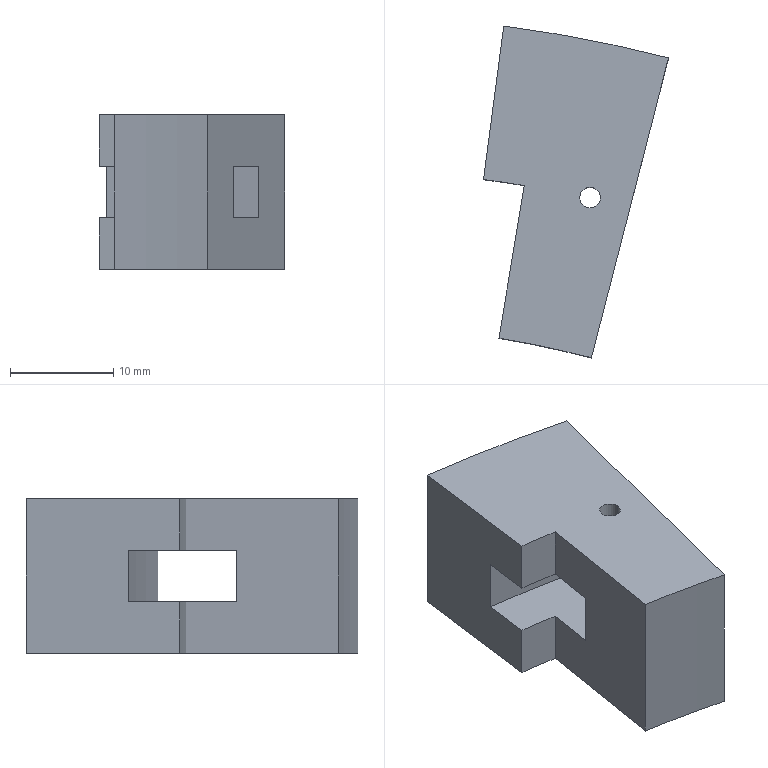Part | SolidWorks | features ICE 5, Extrusion 1 | 1 solid | 17 faces | box 17.933 x 32.148 x 15 mm | volume 5012 mm3 | cylinder 10 | plane 7 | commonest cylinder face diameters 2 x4 240 x2 210 x1 230 x1 249.998 x1 270 x1
STEP:
#1=CARTESIAN_POINT('',(24.989,117.22,0.));
#2=VERTEX_POINT('',#1);
#3=CARTESIAN_POINT('',(26.989,117.22,0.));
#4=VERTEX_POINT('',#3);
#5=CARTESIAN_POINT('',(25.989,117.22,0.));
#6=DIRECTION('',(0.,0.,1.));
#7=DIRECTION('',(1.,0.,0.));
#8=AXIS2_PLACEMENT_3D('',#5,#6,#7);
#9=CIRCLE('',#8,1.);
#10=EDGE_CURVE('',#2,#4,#9,.T.);
#11=ORIENTED_EDGE('',*,*,#10,.F.);
#12=CARTESIAN_POINT('',(24.989,117.22,5.));
#13=VERTEX_POINT('',#12);
#14=CARTESIAN_POINT('',(24.989,117.22,0.));
#15=DIRECTION('',(0.,0.,1.));
#16=VECTOR('',#15,1000.);
#17=LINE('',#14,#16);
#18=EDGE_CURVE('',#2,#13,#17,.T.);
#19=ORIENTED_EDGE('',*,*,#18,.T.);
#20=CARTESIAN_POINT('',(26.989,117.22,5.));
#21=VERTEX_POINT('',#20);
#22=CARTESIAN_POINT('',(25.989,117.22,5.));
#23=DIRECTION('',(0.,0.,1.));
#24=DIRECTION('',(1.,0.,0.));
#25=AXIS2_PLACEMENT_3D('',#22,#23,#24);
#26=CIRCLE('',#25,1.);
#27=EDGE_CURVE('',#13,#21,#26,.T.);
#28=ORIENTED_EDGE('',*,*,#27,.T.);
#29=CARTESIAN_POINT('',(26.989,117.22,0.));
#30=DIRECTION('',(0.,0.,1.));
#31=VECTOR('',#30,1000.);
#32=LINE('',#29,#31);
#33=EDGE_CURVE('',#4,#21,#32,.T.);
#34=ORIENTED_EDGE('',*,*,#33,.F.);
#35=EDGE_LOOP('',(#11,#19,#28,#34));
#36=FACE_OUTER_BOUND('',#35,.T.);
#37=CARTESIAN_POINT('',(25.989,117.22,0.));
#38=DIRECTION('',(0.,0.,1.));
#39=DIRECTION('',(1.,0.,0.));
#40=AXIS2_PLACEMENT_3D('',#37,#38,#39);
#41=CYLINDRICAL_SURFACE('',#40,1.);
#42=ADVANCED_FACE('',(#36),#41,.F.);
#43=CARTESIAN_POINT('',(24.989,117.22,10.));
#44=VERTEX_POINT('',#43);
#45=CARTESIAN_POINT('',(26.989,117.22,10.));
#46=VERTEX_POINT('',#45);
#47=CARTESIAN_POINT('',(25.989,117.22,10.));
#48=DIRECTION('',(0.,0.,1.));
#49=DIRECTION('',(1.,0.,0.));
#50=AXIS2_PLACEMENT_3D('',#47,#48,#49);
#51=CIRCLE('',#50,1.);
#52=EDGE_CURVE('',#44,#46,#51,.T.);
#53=ORIENTED_EDGE('',*,*,#52,.F.);
#54=CARTESIAN_POINT('',(24.989,117.22,15.));
#55=VERTEX_POINT('',#54);
#56=CARTESIAN_POINT('',(24.989,117.22,0.));
#57=DIRECTION('',(0.,0.,1.));
#58=VECTOR('',#57,1000.);
#59=LINE('',#56,#58);
#60=EDGE_CURVE('',#44,#55,#59,.T.);
#61=ORIENTED_EDGE('',*,*,#60,.T.);
#62=CARTESIAN_POINT('',(26.989,117.22,15.));
#63=VERTEX_POINT('',#62);
#64=CARTESIAN_POINT('',(25.989,117.22,15.));
#65=DIRECTION('',(0.,0.,1.));
#66=DIRECTION('',(1.,0.,0.));
#67=AXIS2_PLACEMENT_3D('',#64,#65,#66);
#68=CIRCLE('',#67,1.);
#69=EDGE_CURVE('',#55,#63,#68,.T.);
#70=ORIENTED_EDGE('',*,*,#69,.T.);
#71=CARTESIAN_POINT('',(26.989,117.22,0.));
#72=DIRECTION('',(0.,0.,1.));
#73=VECTOR('',#72,1000.);
#74=LINE('',#71,#73);
#75=EDGE_CURVE('',#46,#63,#74,.T.);
#76=ORIENTED_EDGE('',*,*,#75,.F.);
#77=EDGE_LOOP('',(#53,#61,#70,#76));
#78=FACE_OUTER_BOUND('',#77,.T.);
#79=CARTESIAN_POINT('',(25.989,117.22,0.));
#80=DIRECTION('',(0.,0.,1.));
#81=DIRECTION('',(1.,0.,0.));
#82=AXIS2_PLACEMENT_3D('',#79,#80,#81);
#83=CYLINDRICAL_SURFACE('',#82,1.);
#84=ADVANCED_FACE('',(#78),#83,.F.);
#85=CARTESIAN_POINT('',(28.619,111.382,10.));
#86=VERTEX_POINT('',#85);
#87=CARTESIAN_POINT('',(18.802,113.453,10.));
#88=VERTEX_POINT('',#87);
#89=CARTESIAN_POINT('',(0.,0.,10.));
#90=DIRECTION('',(0.,0.,1.));
#91=DIRECTION('',(1.,0.,0.));
#92=AXIS2_PLACEMENT_3D('',#89,#90,#91);
#93=CIRCLE('',#92,115.);
#94=EDGE_CURVE('',#86,#88,#93,.T.);
#95=ORIENTED_EDGE('',*,*,#94,.F.);
#96=CARTESIAN_POINT('',(28.619,111.382,5.));
#97=VERTEX_POINT('',#96);
#98=CARTESIAN_POINT('',(28.619,111.382,5.));
#99=DIRECTION('',(0.,0.,1.));
#100=VECTOR('',#99,1000.);
#101=LINE('',#98,#100);
#102=EDGE_CURVE('',#97,#86,#101,.T.);
#103=ORIENTED_EDGE('',*,*,#102,.F.);
#104=CARTESIAN_POINT('',(18.802,113.453,5.));
#105=VERTEX_POINT('',#104);
#106=CARTESIAN_POINT('',(0.,0.,5.));
#107=DIRECTION('',(0.,0.,-1.));
#108=DIRECTION('',(1.,0.,0.));
#109=AXIS2_PLACEMENT_3D('',#106,#107,#108);
#110=CIRCLE('',#109,115.);
#111=EDGE_CURVE('',#105,#97,#110,.T.);
#112=ORIENTED_EDGE('',*,*,#111,.F.);
#113=CARTESIAN_POINT('',(18.802,113.453,15.));
#114=DIRECTION('',(0.,0.,-1.));
#115=VECTOR('',#114,1000.);
#116=LINE('',#113,#115);
#117=EDGE_CURVE('',#88,#105,#116,.T.);
#118=ORIENTED_EDGE('',*,*,#117,.F.);
#119=EDGE_LOOP('',(#95,#103,#112,#118));
#120=FACE_OUTER_BOUND('',#119,.T.);
#121=CARTESIAN_POINT('',(0.,0.,5.));
#122=DIRECTION('',(0.,0.,1.));
#123=DIRECTION('',(1.,0.,0.));
#124=AXIS2_PLACEMENT_3D('',#121,#122,#123);
#125=CYLINDRICAL_SURFACE('',#124,115.);
#126=ADVANCED_FACE('',(#120),#125,.T.);
#127=CARTESIAN_POINT('',(16.316,123.93,5.));
#128=VERTEX_POINT('',#127);
#129=CARTESIAN_POINT('',(16.316,123.93,10.));
#130=VERTEX_POINT('',#129);
#131=CARTESIAN_POINT('',(16.316,123.93,5.));
#132=DIRECTION('',(0.,0.,1.));
#133=VECTOR('',#132,1000.);
#134=LINE('',#131,#133);
#135=EDGE_CURVE('',#128,#130,#134,.T.);
#136=ORIENTED_EDGE('',*,*,#135,.F.);
#137=CARTESIAN_POINT('',(31.107,121.067,5.));
#138=VERTEX_POINT('',#137);
#139=CARTESIAN_POINT('',(0.,0.,5.));
#140=DIRECTION('',(0.,0.,-1.));
#141=DIRECTION('',(1.,0.,0.));
#142=AXIS2_PLACEMENT_3D('',#139,#140,#141);
#143=CIRCLE('',#142,124.999);
#144=EDGE_CURVE('',#128,#138,#143,.T.);
#145=ORIENTED_EDGE('',*,*,#144,.T.);
#146=CARTESIAN_POINT('',(31.107,121.067,10.));
#147=VERTEX_POINT('',#146);
#148=CARTESIAN_POINT('',(31.107,121.067,5.));
#149=DIRECTION('',(0.,0.,1.));
#150=VECTOR('',#149,1000.);
#151=LINE('',#148,#150);
#152=EDGE_CURVE('',#138,#147,#151,.T.);
#153=ORIENTED_EDGE('',*,*,#152,.T.);
#154=CARTESIAN_POINT('',(0.,0.,10.));
#155=DIRECTION('',(0.,0.,-1.));
#156=DIRECTION('',(1.,0.,0.));
#157=AXIS2_PLACEMENT_3D('',#154,#155,#156);
#158=CIRCLE('',#157,124.999);
#159=EDGE_CURVE('',#130,#147,#158,.T.);
#160=ORIENTED_EDGE('',*,*,#159,.F.);
#161=EDGE_LOOP('',(#136,#145,#153,#160));
#162=FACE_OUTER_BOUND('',#161,.T.);
#163=CARTESIAN_POINT('',(0.,0.,5.));
#164=DIRECTION('',(0.,0.,1.));
#165=DIRECTION('',(1.,0.,0.));
#166=AXIS2_PLACEMENT_3D('',#163,#164,#165);
#167=CYLINDRICAL_SURFACE('',#166,124.999);
#168=ADVANCED_FACE('',(#162),#167,.F.);
#169=CARTESIAN_POINT('',(33.596,130.753,15.));
#170=VERTEX_POINT('',#169);
#171=CARTESIAN_POINT('',(33.596,130.753,0.));
#172=VERTEX_POINT('',#171);
#173=CARTESIAN_POINT('',(33.596,130.753,15.));
#174=DIRECTION('',(0.,0.,-1.));
#175=VECTOR('',#174,1000.);
#176=LINE('',#173,#175);
#177=EDGE_CURVE('',#170,#172,#176,.T.);
#178=ORIENTED_EDGE('',*,*,#177,.F.);
#179=CARTESIAN_POINT('',(26.13,101.697,15.));
#180=VERTEX_POINT('',#179);
#181=CARTESIAN_POINT('',(26.13,101.697,15.));
#182=DIRECTION('',(0.2489,0.9685,0.));
#183=VECTOR('',#182,1000.);
#184=LINE('',#181,#183);
#185=EDGE_CURVE('',#180,#170,#184,.T.);
#186=ORIENTED_EDGE('',*,*,#185,.F.);
#187=CARTESIAN_POINT('',(26.13,101.697,0.));
#188=VERTEX_POINT('',#187);
#189=CARTESIAN_POINT('',(26.13,101.697,15.));
#190=DIRECTION('',(0.,0.,-1.));
#191=VECTOR('',#190,1000.);
#192=LINE('',#189,#191);
#193=EDGE_CURVE('',#180,#188,#192,.T.);
#194=ORIENTED_EDGE('',*,*,#193,.T.);
#195=CARTESIAN_POINT('',(26.13,101.697,0.));
#196=DIRECTION('',(0.2489,0.9685,0.));
#197=VECTOR('',#196,1000.);
#198=LINE('',#195,#197);
#199=EDGE_CURVE('',#188,#172,#198,.T.);
#200=ORIENTED_EDGE('',*,*,#199,.T.);
#201=EDGE_LOOP('',(#178,#186,#194,#200));
#202=FACE_OUTER_BOUND('',#201,.T.);
#203=ORIENTED_EDGE('',*,*,#152,.F.);
#204=CARTESIAN_POINT('',(0.,0.,5.));
#205=DIRECTION('',(0.2489,0.9685,0.));
#206=VECTOR('',#205,1000.);
#207=LINE('',#204,#206);
#208=EDGE_CURVE('',#97,#138,#207,.T.);
#209=ORIENTED_EDGE('',*,*,#208,.F.);
#210=ORIENTED_EDGE('',*,*,#102,.T.);
#211=CARTESIAN_POINT('',(0.,0.,10.));
#212=DIRECTION('',(0.2489,0.9685,0.));
#213=VECTOR('',#212,1000.);
#214=LINE('',#211,#213);
#215=EDGE_CURVE('',#86,#147,#214,.T.);
#216=ORIENTED_EDGE('',*,*,#215,.T.);
#217=EDGE_LOOP('',(#203,#209,#210,#216));
#218=FACE_BOUND('',#217,.T.);
#219=CARTESIAN_POINT('',(26.13,101.697,15.));
#220=DIRECTION('',(-0.9685,0.2489,0.));
#221=DIRECTION('',(-0.2489,-0.9685,0.));
#222=AXIS2_PLACEMENT_3D('',#219,#220,#221);
#223=PLANE('',#222);
#224=ADVANCED_FACE('',(#202,#218),#223,.F.);
#225=CARTESIAN_POINT('',(17.621,133.845,0.));
#226=VERTEX_POINT('',#225);
#227=CARTESIAN_POINT('',(0.,0.,0.));
#228=DIRECTION('',(0.,0.,1.));
#229=DIRECTION('',(1.,0.,0.));
#230=AXIS2_PLACEMENT_3D('',#227,#228,#229);
#231=CIRCLE('',#230,135.);
#232=EDGE_CURVE('',#172,#226,#231,.T.);
#233=ORIENTED_EDGE('',*,*,#232,.T.);
#234=CARTESIAN_POINT('',(17.621,133.845,15.));
#235=VERTEX_POINT('',#234);
#236=CARTESIAN_POINT('',(17.621,133.845,0.));
#237=DIRECTION('',(0.,0.,1.));
#238=VECTOR('',#237,1000.);
#239=LINE('',#236,#238);
#240=EDGE_CURVE('',#226,#235,#239,.T.);
#241=ORIENTED_EDGE('',*,*,#240,.T.);
#242=CARTESIAN_POINT('',(0.,0.,15.));
#243=DIRECTION('',(0.,0.,1.));
#244=DIRECTION('',(1.,0.,0.));
#245=AXIS2_PLACEMENT_3D('',#242,#243,#244);
#246=CIRCLE('',#245,135.);
#247=EDGE_CURVE('',#170,#235,#246,.T.);
#248=ORIENTED_EDGE('',*,*,#247,.F.);
#249=ORIENTED_EDGE('',*,*,#177,.T.);
#250=EDGE_LOOP('',(#233,#241,#248,#249));
#251=FACE_OUTER_BOUND('',#250,.T.);
#252=CARTESIAN_POINT('',(0.,0.,15.));
#253=DIRECTION('',(0.,0.,-1.));
#254=DIRECTION('',(-1.,0.,0.));
#255=AXIS2_PLACEMENT_3D('',#252,#253,#254);
#256=CYLINDRICAL_SURFACE('',#255,135.);
#257=ADVANCED_FACE('',(#251),#256,.T.);
#258=CARTESIAN_POINT('',(19.62,118.385,0.));
#259=VERTEX_POINT('',#258);
#260=CARTESIAN_POINT('',(17.167,103.587,0.));
#261=VERTEX_POINT('',#260);
#262=CARTESIAN_POINT('',(17.167,103.587,0.));
#263=DIRECTION('',(-0.1635,-0.9865,0.));
#264=VECTOR('',#263,1000.);
#265=LINE('',#262,#264);
#266=EDGE_CURVE('',#259,#261,#265,.T.);
#267=ORIENTED_EDGE('',*,*,#266,.T.);
#268=CARTESIAN_POINT('',(17.167,103.587,15.));
#269=VERTEX_POINT('',#268);
#270=CARTESIAN_POINT('',(17.167,103.587,15.));
#271=DIRECTION('',(0.,0.,-1.));
#272=VECTOR('',#271,1000.);
#273=LINE('',#270,#272);
#274=EDGE_CURVE('',#269,#261,#273,.T.);
#275=ORIENTED_EDGE('',*,*,#274,.F.);
#276=CARTESIAN_POINT('',(19.62,118.385,15.));
#277=VERTEX_POINT('',#276);
#278=CARTESIAN_POINT('',(17.167,103.587,15.));
#279=DIRECTION('',(-0.1635,-0.9865,0.));
#280=VECTOR('',#279,1000.);
#281=LINE('',#278,#280);
#282=EDGE_CURVE('',#277,#269,#281,.T.);
#283=ORIENTED_EDGE('',*,*,#282,.F.);
#284=CARTESIAN_POINT('',(19.62,118.385,10.));
#285=VERTEX_POINT('',#284);
#286=CARTESIAN_POINT('',(19.62,118.385,0.));
#287=DIRECTION('',(0.,0.,1.));
#288=VECTOR('',#287,1000.);
#289=LINE('',#286,#288);
#290=EDGE_CURVE('',#285,#277,#289,.T.);
#291=ORIENTED_EDGE('',*,*,#290,.F.);
#292=CARTESIAN_POINT('',(0.,0.,10.));
#293=DIRECTION('',(0.1635,0.9865,0.));
#294=VECTOR('',#293,1000.);
#295=LINE('',#292,#294);
#296=EDGE_CURVE('',#88,#285,#295,.T.);
#297=ORIENTED_EDGE('',*,*,#296,.F.);
#298=ORIENTED_EDGE('',*,*,#117,.T.);
#299=CARTESIAN_POINT('',(19.62,118.385,5.));
#300=VERTEX_POINT('',#299);
#301=CARTESIAN_POINT('',(0.,0.,5.));
#302=DIRECTION('',(0.1635,0.9865,0.));
#303=VECTOR('',#302,1000.);
#304=LINE('',#301,#303);
#305=EDGE_CURVE('',#105,#300,#304,.T.);
#306=ORIENTED_EDGE('',*,*,#305,.T.);
#307=CARTESIAN_POINT('',(19.62,118.385,0.));
#308=DIRECTION('',(0.,0.,1.));
#309=VECTOR('',#308,1000.);
#310=LINE('',#307,#309);
#311=EDGE_CURVE('',#259,#300,#310,.T.);
#312=ORIENTED_EDGE('',*,*,#311,.F.);
#313=EDGE_LOOP('',(#267,#275,#283,#291,#297,#298,#306,#312));
#314=FACE_OUTER_BOUND('',#313,.T.);
#315=CARTESIAN_POINT('',(17.167,103.587,15.));
#316=DIRECTION('',(0.9865,-0.1635,0.));
#317=DIRECTION('',(0.1635,0.9865,0.));
#318=AXIS2_PLACEMENT_3D('',#315,#316,#317);
#319=PLANE('',#318);
#320=ADVANCED_FACE('',(#314),#319,.F.);
#321=CARTESIAN_POINT('',(0.,0.,0.));
#322=DIRECTION('',(0.,0.,-1.));
#323=DIRECTION('',(1.,0.,0.));
#324=AXIS2_PLACEMENT_3D('',#321,#322,#323);
#325=CIRCLE('',#324,105.);
#326=EDGE_CURVE('',#261,#188,#325,.T.);
#327=ORIENTED_EDGE('',*,*,#326,.T.);
#328=ORIENTED_EDGE('',*,*,#193,.F.);
#329=CARTESIAN_POINT('',(0.,0.,15.));
#330=DIRECTION('',(0.,0.,-1.));
#331=DIRECTION('',(1.,0.,0.));
#332=AXIS2_PLACEMENT_3D('',#329,#330,#331);
#333=CIRCLE('',#332,105.);
#334=EDGE_CURVE('',#269,#180,#333,.T.);
#335=ORIENTED_EDGE('',*,*,#334,.F.);
#336=ORIENTED_EDGE('',*,*,#274,.T.);
#337=EDGE_LOOP('',(#327,#328,#335,#336));
#338=FACE_OUTER_BOUND('',#337,.T.);
#339=CARTESIAN_POINT('',(0.,0.,15.));
#340=DIRECTION('',(0.,0.,-1.));
#341=DIRECTION('',(-1.,0.,0.));
#342=AXIS2_PLACEMENT_3D('',#339,#340,#341);
#343=CYLINDRICAL_SURFACE('',#342,105.);
#344=ADVANCED_FACE('',(#338),#343,.F.);
#345=CARTESIAN_POINT('',(15.663,118.973,15.));
#346=VERTEX_POINT('',#345);
#347=CARTESIAN_POINT('',(0.,0.,15.));
#348=DIRECTION('',(0.,0.,1.));
#349=DIRECTION('',(1.,0.,0.));
#350=AXIS2_PLACEMENT_3D('',#347,#348,#349);
#351=CIRCLE('',#350,120.);
#352=EDGE_CURVE('',#277,#346,#351,.T.);
#353=ORIENTED_EDGE('',*,*,#352,.F.);
#354=ORIENTED_EDGE('',*,*,#282,.T.);
#355=ORIENTED_EDGE('',*,*,#334,.T.);
#356=ORIENTED_EDGE('',*,*,#185,.T.);
#357=ORIENTED_EDGE('',*,*,#247,.T.);
#358=CARTESIAN_POINT('',(15.011,114.016,15.));
#359=DIRECTION('',(0.1305,0.9914,0.));
#360=VECTOR('',#359,1000.);
#361=LINE('',#358,#360);
#362=EDGE_CURVE('',#346,#235,#361,.T.);
#363=ORIENTED_EDGE('',*,*,#362,.F.);
#364=EDGE_LOOP('',(#353,#354,#355,#356,#357,#363));
#365=FACE_OUTER_BOUND('',#364,.T.);
#366=CARTESIAN_POINT('',(25.989,117.22,15.));
#367=DIRECTION('',(0.,0.,1.));
#368=DIRECTION('',(1.,0.,0.));
#369=AXIS2_PLACEMENT_3D('',#366,#367,#368);
#370=CIRCLE('',#369,1.);
#371=EDGE_CURVE('',#63,#55,#370,.T.);
#372=ORIENTED_EDGE('',*,*,#371,.F.);
#373=ORIENTED_EDGE('',*,*,#69,.F.);
#374=EDGE_LOOP('',(#372,#373));
#375=FACE_BOUND('',#374,.T.);
#376=CARTESIAN_POINT('',(0.,0.,15.));
#377=DIRECTION('',(0.,0.,1.));
#378=DIRECTION('',(1.,0.,0.));
#379=AXIS2_PLACEMENT_3D('',#376,#377,#378);
#380=PLANE('',#379);
#381=ADVANCED_FACE('',(#365,#375),#380,.T.);
#382=CARTESIAN_POINT('',(25.989,117.22,0.));
#383=DIRECTION('',(0.,0.,1.));
#384=DIRECTION('',(1.,0.,0.));
#385=AXIS2_PLACEMENT_3D('',#382,#383,#384);
#386=CIRCLE('',#385,1.);
#387=EDGE_CURVE('',#4,#2,#386,.T.);
#388=ORIENTED_EDGE('',*,*,#387,.T.);
#389=ORIENTED_EDGE('',*,*,#10,.T.);
#390=EDGE_LOOP('',(#388,#389));
#391=FACE_BOUND('',#390,.T.);
#392=ORIENTED_EDGE('',*,*,#266,.F.);
#393=CARTESIAN_POINT('',(15.663,118.973,0.));
#394=VERTEX_POINT('',#393);
#395=CARTESIAN_POINT('',(0.,0.,0.));
#396=DIRECTION('',(0.,0.,1.));
#397=DIRECTION('',(1.,0.,0.));
#398=AXIS2_PLACEMENT_3D('',#395,#396,#397);
#399=CIRCLE('',#398,120.);
#400=EDGE_CURVE('',#259,#394,#399,.T.);
#401=ORIENTED_EDGE('',*,*,#400,.T.);
#402=CARTESIAN_POINT('',(15.011,114.016,0.));
#403=DIRECTION('',(0.1305,0.9914,0.));
#404=VECTOR('',#403,1000.);
#405=LINE('',#402,#404);
#406=EDGE_CURVE('',#394,#226,#405,.T.);
#407=ORIENTED_EDGE('',*,*,#406,.T.);
#408=ORIENTED_EDGE('',*,*,#232,.F.);
#409=ORIENTED_EDGE('',*,*,#199,.F.);
#410=ORIENTED_EDGE('',*,*,#326,.F.);
#411=EDGE_LOOP('',(#392,#401,#407,#408,#409,#410));
#412=FACE_OUTER_BOUND('',#411,.T.);
#413=CARTESIAN_POINT('',(0.,0.,0.));
#414=DIRECTION('',(0.,0.,1.));
#415=DIRECTION('',(1.,0.,0.));
#416=AXIS2_PLACEMENT_3D('',#413,#414,#415);
#417=PLANE('',#416);
#418=ADVANCED_FACE('',(#391,#412),#417,.F.);
#419=CARTESIAN_POINT('',(15.663,118.973,5.));
#420=VERTEX_POINT('',#419);
#421=CARTESIAN_POINT('',(0.,0.,5.));
#422=DIRECTION('',(0.,0.,1.));
#423=DIRECTION('',(1.,0.,0.));
#424=AXIS2_PLACEMENT_3D('',#421,#422,#423);
#425=CIRCLE('',#424,120.);
#426=EDGE_CURVE('',#300,#420,#425,.T.);
#427=ORIENTED_EDGE('',*,*,#426,.F.);
#428=ORIENTED_EDGE('',*,*,#305,.F.);
#429=ORIENTED_EDGE('',*,*,#111,.T.);
#430=ORIENTED_EDGE('',*,*,#208,.T.);
#431=ORIENTED_EDGE('',*,*,#144,.F.);
#432=CARTESIAN_POINT('',(0.,0.,5.));
#433=DIRECTION('',(0.1305,0.9914,0.));
#434=VECTOR('',#433,1000.);
#435=LINE('',#432,#434);
#436=EDGE_CURVE('',#420,#128,#435,.T.);
#437=ORIENTED_EDGE('',*,*,#436,.F.);
#438=EDGE_LOOP('',(#427,#428,#429,#430,#431,#437));
#439=FACE_OUTER_BOUND('',#438,.T.);
#440=CARTESIAN_POINT('',(25.989,117.22,5.));
#441=DIRECTION('',(0.,0.,1.));
#442=DIRECTION('',(1.,0.,0.));
#443=AXIS2_PLACEMENT_3D('',#440,#441,#442);
#444=CIRCLE('',#443,1.);
#445=EDGE_CURVE('',#21,#13,#444,.T.);
#446=ORIENTED_EDGE('',*,*,#445,.F.);
#447=ORIENTED_EDGE('',*,*,#27,.F.);
#448=EDGE_LOOP('',(#446,#447));
#449=FACE_BOUND('',#448,.T.);
#450=CARTESIAN_POINT('',(0.,0.,5.));
#451=DIRECTION('',(0.,0.,1.));
#452=DIRECTION('',(1.,0.,0.));
#453=AXIS2_PLACEMENT_3D('',#450,#451,#452);
#454=PLANE('',#453);
#455=ADVANCED_FACE('',(#439,#449),#454,.T.);
#456=CARTESIAN_POINT('',(25.989,117.22,10.));
#457=DIRECTION('',(0.,0.,1.));
#458=DIRECTION('',(1.,0.,0.));
#459=AXIS2_PLACEMENT_3D('',#456,#457,#458);
#460=CIRCLE('',#459,1.);
#461=EDGE_CURVE('',#46,#44,#460,.T.);
#462=ORIENTED_EDGE('',*,*,#461,.T.);
#463=ORIENTED_EDGE('',*,*,#52,.T.);
#464=EDGE_LOOP('',(#462,#463));
#465=FACE_BOUND('',#464,.T.);
#466=ORIENTED_EDGE('',*,*,#296,.T.);
#467=CARTESIAN_POINT('',(15.663,118.973,10.));
#468=VERTEX_POINT('',#467);
#469=CARTESIAN_POINT('',(0.,0.,10.));
#470=DIRECTION('',(0.,0.,1.));
#471=DIRECTION('',(1.,0.,0.));
#472=AXIS2_PLACEMENT_3D('',#469,#470,#471);
#473=CIRCLE('',#472,120.);
#474=EDGE_CURVE('',#285,#468,#473,.T.);
#475=ORIENTED_EDGE('',*,*,#474,.T.);
#476=CARTESIAN_POINT('',(0.,0.,10.));
#477=DIRECTION('',(0.1305,0.9914,0.));
#478=VECTOR('',#477,1000.);
#479=LINE('',#476,#478);
#480=EDGE_CURVE('',#468,#130,#479,.T.);
#481=ORIENTED_EDGE('',*,*,#480,.T.);
#482=ORIENTED_EDGE('',*,*,#159,.T.);
#483=ORIENTED_EDGE('',*,*,#215,.F.);
#484=ORIENTED_EDGE('',*,*,#94,.T.);
#485=EDGE_LOOP('',(#466,#475,#481,#482,#483,#484));
#486=FACE_OUTER_BOUND('',#485,.T.);
#487=CARTESIAN_POINT('',(0.,0.,10.));
#488=DIRECTION('',(0.,0.,1.));
#489=DIRECTION('',(1.,0.,0.));
#490=AXIS2_PLACEMENT_3D('',#487,#488,#489);
#491=PLANE('',#490);
#492=ADVANCED_FACE('',(#465,#486),#491,.F.);
#493=ORIENTED_EDGE('',*,*,#60,.F.);
#494=ORIENTED_EDGE('',*,*,#461,.F.);
#495=ORIENTED_EDGE('',*,*,#75,.T.);
#496=ORIENTED_EDGE('',*,*,#371,.T.);
#497=EDGE_LOOP('',(#493,#494,#495,#496));
#498=FACE_OUTER_BOUND('',#497,.T.);
#499=CARTESIAN_POINT('',(25.989,117.22,0.));
#500=DIRECTION('',(0.,0.,1.));
#501=DIRECTION('',(1.,0.,0.));
#502=AXIS2_PLACEMENT_3D('',#499,#500,#501);
#503=CYLINDRICAL_SURFACE('',#502,1.);
#504=ADVANCED_FACE('',(#498),#503,.F.);
#505=ORIENTED_EDGE('',*,*,#18,.F.);
#506=ORIENTED_EDGE('',*,*,#387,.F.);
#507=ORIENTED_EDGE('',*,*,#33,.T.);
#508=ORIENTED_EDGE('',*,*,#445,.T.);
#509=EDGE_LOOP('',(#505,#506,#507,#508));
#510=FACE_OUTER_BOUND('',#509,.T.);
#511=CARTESIAN_POINT('',(25.989,117.22,0.));
#512=DIRECTION('',(0.,0.,1.));
#513=DIRECTION('',(1.,0.,0.));
#514=AXIS2_PLACEMENT_3D('',#511,#512,#513);
#515=CYLINDRICAL_SURFACE('',#514,1.);
#516=ADVANCED_FACE('',(#510),#515,.F.);
#517=ORIENTED_EDGE('',*,*,#406,.F.);
#518=CARTESIAN_POINT('',(15.663,118.973,0.));
#519=DIRECTION('',(0.,0.,1.));
#520=VECTOR('',#519,1000.);
#521=LINE('',#518,#520);
#522=EDGE_CURVE('',#394,#420,#521,.T.);
#523=ORIENTED_EDGE('',*,*,#522,.T.);
#524=ORIENTED_EDGE('',*,*,#436,.T.);
#525=ORIENTED_EDGE('',*,*,#135,.T.);
#526=ORIENTED_EDGE('',*,*,#480,.F.);
#527=CARTESIAN_POINT('',(15.663,118.973,0.));
#528=DIRECTION('',(0.,0.,1.));
#529=VECTOR('',#528,1000.);
#530=LINE('',#527,#529);
#531=EDGE_CURVE('',#468,#346,#530,.T.);
#532=ORIENTED_EDGE('',*,*,#531,.T.);
#533=ORIENTED_EDGE('',*,*,#362,.T.);
#534=ORIENTED_EDGE('',*,*,#240,.F.);
#535=EDGE_LOOP('',(#517,#523,#524,#525,#526,#532,#533,#534));
#536=FACE_OUTER_BOUND('',#535,.T.);
#537=CARTESIAN_POINT('',(15.011,114.016,0.));
#538=DIRECTION('',(0.9914,-0.1305,0.));
#539=DIRECTION('',(0.1305,0.9914,0.));
#540=AXIS2_PLACEMENT_3D('',#537,#538,#539);
#541=PLANE('',#540);
#542=ADVANCED_FACE('',(#536),#541,.F.);
#543=ORIENTED_EDGE('',*,*,#290,.T.);
#544=ORIENTED_EDGE('',*,*,#352,.T.);
#545=ORIENTED_EDGE('',*,*,#531,.F.);
#546=ORIENTED_EDGE('',*,*,#474,.F.);
#547=EDGE_LOOP('',(#543,#544,#545,#546));
#548=FACE_OUTER_BOUND('',#547,.T.);
#549=CARTESIAN_POINT('',(0.,0.,0.));
#550=DIRECTION('',(0.,0.,1.));
#551=DIRECTION('',(1.,0.,0.));
#552=AXIS2_PLACEMENT_3D('',#549,#550,#551);
#553=CYLINDRICAL_SURFACE('',#552,120.);
#554=ADVANCED_FACE('',(#548),#553,.F.);
#555=ORIENTED_EDGE('',*,*,#426,.T.);
#556=ORIENTED_EDGE('',*,*,#522,.F.);
#557=ORIENTED_EDGE('',*,*,#400,.F.);
#558=ORIENTED_EDGE('',*,*,#311,.T.);
#559=EDGE_LOOP('',(#555,#556,#557,#558));
#560=FACE_OUTER_BOUND('',#559,.T.);
#561=CARTESIAN_POINT('',(0.,0.,0.));
#562=DIRECTION('',(0.,0.,1.));
#563=DIRECTION('',(1.,0.,0.));
#564=AXIS2_PLACEMENT_3D('',#561,#562,#563);
#565=CYLINDRICAL_SURFACE('',#564,120.);
#566=ADVANCED_FACE('',(#560),#565,.F.);
#567=CLOSED_SHELL('',(#42,#84,#126,#168,#224,#257,#320,#344,#381,#418,#455,#492,#504,#516,#542,#554,#566));
#568=MANIFOLD_SOLID_BREP('',#567);
#569=CARTESIAN_POINT('',(0.,0.,0.));
#570=DIRECTION('',(0.,0.,1.));
#571=DIRECTION('',(1.,0.,0.));
#572=AXIS2_PLACEMENT_3D('',#569,#570,#571);
#573=(LENGTH_UNIT()NAMED_UNIT(*)SI_UNIT(.MILLI.,.METRE.));
#574=UNCERTAINTY_MEASURE_WITH_UNIT(LENGTH_MEASURE(0.00001),#573,'','');
#575=(NAMED_UNIT(*)PLANE_ANGLE_UNIT()SI_UNIT($,.RADIAN.));
#576=(NAMED_UNIT(*)SI_UNIT($,.STERADIAN.)SOLID_ANGLE_UNIT());
#577=(GEOMETRIC_REPRESENTATION_CONTEXT(3)GLOBAL_UNCERTAINTY_ASSIGNED_CONTEXT((#574))GLOBAL_UNIT_ASSIGNED_CONTEXT((#573,#575,#576))REPRESENTATION_CONTEXT('',''));
#578=ADVANCED_BREP_SHAPE_REPRESENTATION('',(#568,#572),#577);